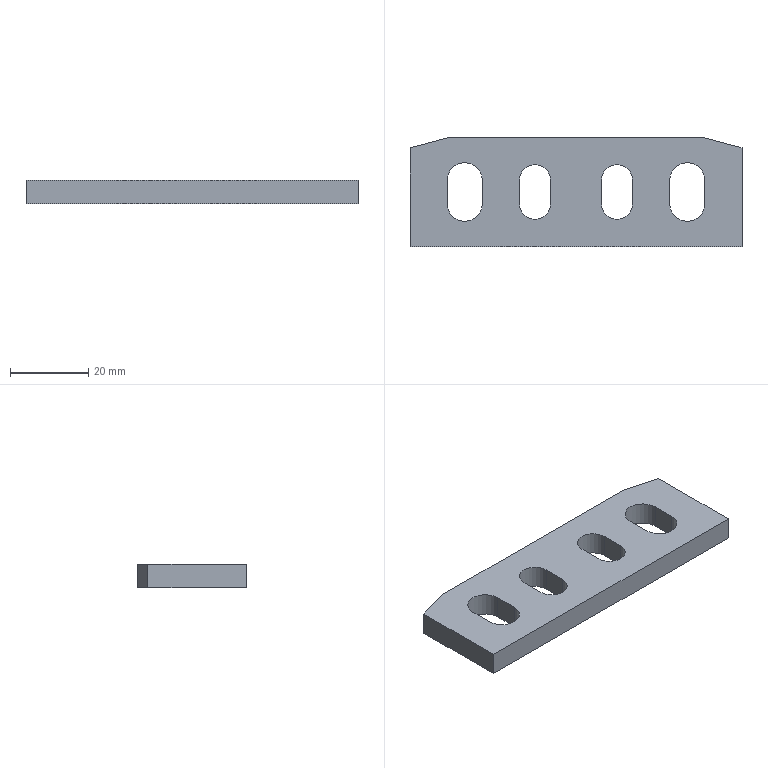Part | STEP file | gslz 2016.10.28-13_id1602_x_t | 1 solid | 24 faces | box 85 x 28 x 6 mm | volume 11529 mm3 | plane 16 | cylinder 8 | commonest cylinder face diameters 8 x4 9 x4